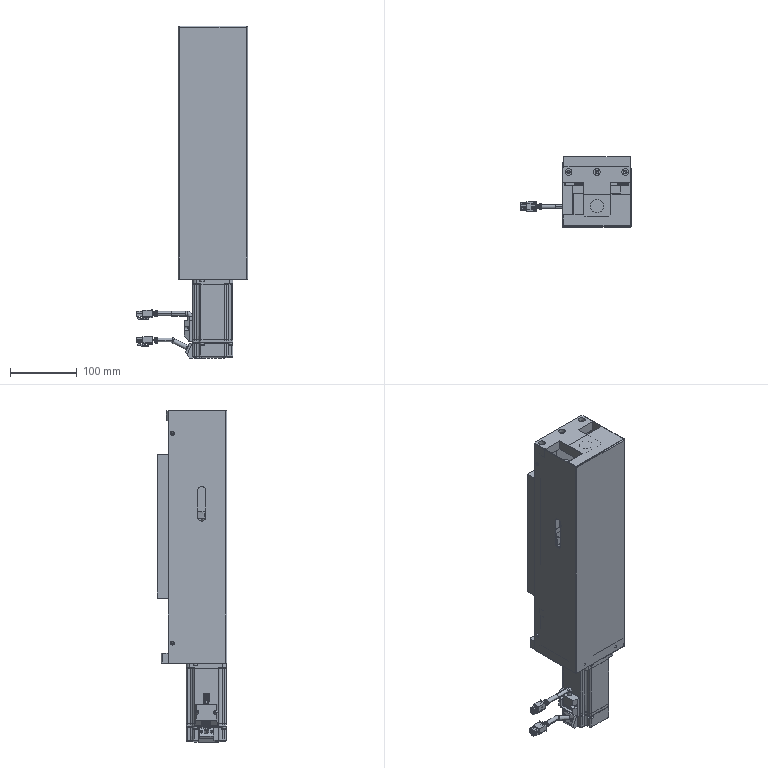Part | SolidWorks | 36 solids | 2723 faces | box 166.8 x 105 x 498.5 mm | volume 1079493 mm3 | plane 1291 | cylinder 789 | spline 327 | cone 272 | torus 36 | sphere 8 | commonest cylinder face diameters 2.5 x92 3 x88 6 x75 4 x41 5.5 x40 0.6 x38